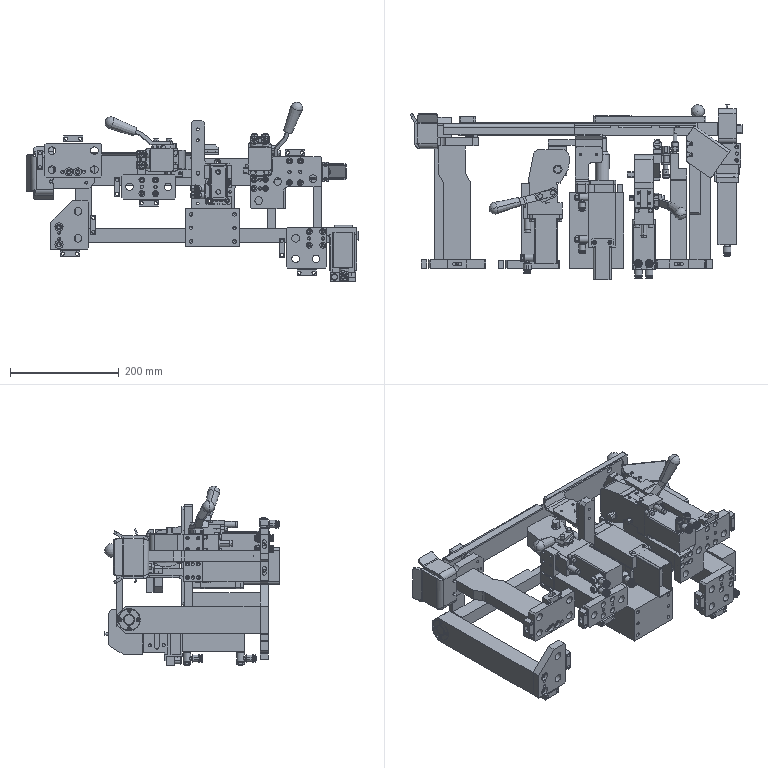Part | NX | features BREP 111 | 111 solids | 3847 faces | volume 6174337 mm3 | plane 1896 | cylinder 1289 | cone 598 | torus 36 | sphere 22 | spline 6 | commonest cylinder face diameters 6 x137 5 x113 10 x67 7 x63 4.134 x52 0.8 x48